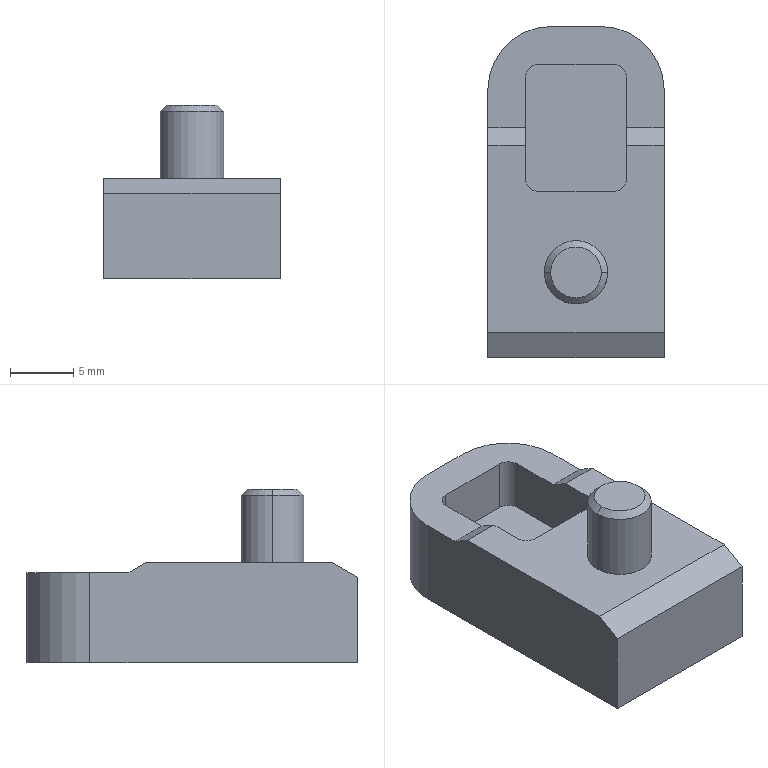Part | SolidWorks | features ICE 4, RefAxis 3, 3DProfileFeature 1, Extrusion 1, RevCut 1, Revolution 1 | 1 solid | 41 faces | box 13.9 x 26.1 x 13.7 mm | volume 2228 mm3 | plane 25 | cylinder 12 | cone 4 | commonest cylinder face diameters 2 x4 10 x4 5 x2 8.5 x2
STEP:
#1=CARTESIAN_POINT('',(2.5,6.7,7.9));
#2=VERTEX_POINT('',#1);
#3=CARTESIAN_POINT('',(-2.5,6.7,7.9));
#4=VERTEX_POINT('',#3);
#5=CARTESIAN_POINT('',(0.,6.7,7.9));
#6=DIRECTION('',(0.,0.,1.));
#7=DIRECTION('',(1.,0.,0.));
#8=AXIS2_PLACEMENT_3D('',#5,#6,#7);
#9=CIRCLE('',#8,2.5);
#10=EDGE_CURVE('',#2,#4,#9,.T.);
#11=ORIENTED_EDGE('',*,*,#10,.T.);
#12=CARTESIAN_POINT('',(-2.5,6.7,13.21));
#13=VERTEX_POINT('',#12);
#14=CARTESIAN_POINT('',(-2.5,6.7,7.9));
#15=DIRECTION('',(0.,0.,1.));
#16=VECTOR('',#15,1000.);
#17=LINE('',#14,#16);
#18=EDGE_CURVE('',#4,#13,#17,.T.);
#19=ORIENTED_EDGE('',*,*,#18,.T.);
#20=CARTESIAN_POINT('',(2.5,6.7,13.21));
#21=VERTEX_POINT('',#20);
#22=CARTESIAN_POINT('',(0.,6.7,13.21));
#23=DIRECTION('',(0.,0.,1.));
#24=DIRECTION('',(1.,0.,0.));
#25=AXIS2_PLACEMENT_3D('',#22,#23,#24);
#26=CIRCLE('',#25,2.5);
#27=EDGE_CURVE('',#21,#13,#26,.T.);
#28=ORIENTED_EDGE('',*,*,#27,.F.);
#29=CARTESIAN_POINT('',(2.5,6.7,7.9));
#30=DIRECTION('',(0.,0.,1.));
#31=VECTOR('',#30,1000.);
#32=LINE('',#29,#31);
#33=EDGE_CURVE('',#2,#21,#32,.T.);
#34=ORIENTED_EDGE('',*,*,#33,.F.);
#35=EDGE_LOOP('',(#11,#19,#28,#34));
#36=FACE_OUTER_BOUND('',#35,.T.);
#37=CARTESIAN_POINT('',(0.,6.7,7.9));
#38=DIRECTION('',(0.,0.,1.));
#39=DIRECTION('',(1.,0.,0.));
#40=AXIS2_PLACEMENT_3D('',#37,#38,#39);
#41=CYLINDRICAL_SURFACE('',#40,2.5);
#42=ADVANCED_FACE('',(#36),#41,.T.);
#43=CARTESIAN_POINT('',(2.01,6.7,13.7));
#44=VERTEX_POINT('',#43);
#45=CARTESIAN_POINT('',(-2.01,6.7,13.7));
#46=VERTEX_POINT('',#45);
#47=CARTESIAN_POINT('',(0.,6.7,13.7));
#48=DIRECTION('',(0.,0.,1.));
#49=DIRECTION('',(1.,0.,0.));
#50=AXIS2_PLACEMENT_3D('',#47,#48,#49);
#51=CIRCLE('',#50,2.01);
#52=EDGE_CURVE('',#44,#46,#51,.T.);
#53=ORIENTED_EDGE('',*,*,#52,.F.);
#54=CARTESIAN_POINT('',(2.5,6.7,13.21));
#55=DIRECTION('',(0.7071,0.,-0.7071));
#56=VECTOR('',#55,1000.);
#57=LINE('',#54,#56);
#58=EDGE_CURVE('',#44,#21,#57,.T.);
#59=ORIENTED_EDGE('',*,*,#58,.T.);
#60=ORIENTED_EDGE('',*,*,#27,.T.);
#61=CARTESIAN_POINT('',(-2.5,6.7,13.21));
#62=DIRECTION('',(-0.7071,0.,-0.7071));
#63=VECTOR('',#62,1000.);
#64=LINE('',#61,#63);
#65=EDGE_CURVE('',#46,#13,#64,.T.);
#66=ORIENTED_EDGE('',*,*,#65,.F.);
#67=EDGE_LOOP('',(#53,#59,#60,#66));
#68=FACE_OUTER_BOUND('',#67,.T.);
#69=CARTESIAN_POINT('',(0.,6.7,13.21));
#70=DIRECTION('',(0.,0.,-1.));
#71=DIRECTION('',(-1.,0.,0.));
#72=AXIS2_PLACEMENT_3D('',#69,#70,#71);
#73=CONICAL_SURFACE('',#72,2.5,0.7854);
#74=ADVANCED_FACE('',(#68),#73,.T.);
#75=CARTESIAN_POINT('',(-5.,6.7,0.));
#76=VERTEX_POINT('',#75);
#77=CARTESIAN_POINT('',(5.,6.7,0.));
#78=VERTEX_POINT('',#77);
#79=CARTESIAN_POINT('',(0.,6.7,0.));
#80=DIRECTION('',(0.,0.,1.));
#81=DIRECTION('',(1.,0.,0.));
#82=AXIS2_PLACEMENT_3D('',#79,#80,#81);
#83=CIRCLE('',#82,5.);
#84=EDGE_CURVE('',#76,#78,#83,.T.);
#85=ORIENTED_EDGE('',*,*,#84,.F.);
#86=CARTESIAN_POINT('',(-5.,6.7,5.7));
#87=VERTEX_POINT('',#86);
#88=CARTESIAN_POINT('',(-5.,6.7,0.));
#89=DIRECTION('',(0.,0.,1.));
#90=VECTOR('',#89,1000.);
#91=LINE('',#88,#90);
#92=EDGE_CURVE('',#76,#87,#91,.T.);
#93=ORIENTED_EDGE('',*,*,#92,.T.);
#94=CARTESIAN_POINT('',(5.,6.7,5.7));
#95=VERTEX_POINT('',#94);
#96=CARTESIAN_POINT('',(0.,6.7,5.7));
#97=DIRECTION('',(0.,0.,1.));
#98=DIRECTION('',(1.,0.,0.));
#99=AXIS2_PLACEMENT_3D('',#96,#97,#98);
#100=CIRCLE('',#99,5.);
#101=EDGE_CURVE('',#87,#95,#100,.T.);
#102=ORIENTED_EDGE('',*,*,#101,.T.);
#103=CARTESIAN_POINT('',(5.,6.7,0.));
#104=DIRECTION('',(0.,0.,1.));
#105=VECTOR('',#104,1000.);
#106=LINE('',#103,#105);
#107=EDGE_CURVE('',#78,#95,#106,.T.);
#108=ORIENTED_EDGE('',*,*,#107,.F.);
#109=EDGE_LOOP('',(#85,#93,#102,#108));
#110=FACE_OUTER_BOUND('',#109,.T.);
#111=CARTESIAN_POINT('',(0.,6.7,0.));
#112=DIRECTION('',(0.,0.,1.));
#113=DIRECTION('',(1.,0.,0.));
#114=AXIS2_PLACEMENT_3D('',#111,#112,#113);
#115=CYLINDRICAL_SURFACE('',#114,5.);
#116=ADVANCED_FACE('',(#110),#115,.F.);
#117=CARTESIAN_POINT('',(4.25,6.7,1.2));
#118=VERTEX_POINT('',#117);
#119=CARTESIAN_POINT('',(-4.25,6.7,1.2));
#120=VERTEX_POINT('',#119);
#121=CARTESIAN_POINT('',(0.,6.7,1.2));
#122=DIRECTION('',(0.,0.,1.));
#123=DIRECTION('',(1.,0.,0.));
#124=AXIS2_PLACEMENT_3D('',#121,#122,#123);
#125=CIRCLE('',#124,4.25);
#126=EDGE_CURVE('',#118,#120,#125,.T.);
#127=ORIENTED_EDGE('',*,*,#126,.T.);
#128=CARTESIAN_POINT('',(-4.25,6.7,5.7));
#129=VERTEX_POINT('',#128);
#130=CARTESIAN_POINT('',(-4.25,6.7,0.));
#131=DIRECTION('',(0.,0.,1.));
#132=VECTOR('',#131,1000.);
#133=LINE('',#130,#132);
#134=EDGE_CURVE('',#120,#129,#133,.T.);
#135=ORIENTED_EDGE('',*,*,#134,.T.);
#136=CARTESIAN_POINT('',(4.25,6.7,5.7));
#137=VERTEX_POINT('',#136);
#138=CARTESIAN_POINT('',(0.,6.7,5.7));
#139=DIRECTION('',(0.,0.,1.));
#140=DIRECTION('',(1.,0.,0.));
#141=AXIS2_PLACEMENT_3D('',#138,#139,#140);
#142=CIRCLE('',#141,4.25);
#143=EDGE_CURVE('',#137,#129,#142,.T.);
#144=ORIENTED_EDGE('',*,*,#143,.F.);
#145=CARTESIAN_POINT('',(4.25,6.7,0.));
#146=DIRECTION('',(0.,0.,1.));
#147=VECTOR('',#146,1000.);
#148=LINE('',#145,#147);
#149=EDGE_CURVE('',#118,#137,#148,.T.);
#150=ORIENTED_EDGE('',*,*,#149,.F.);
#151=EDGE_LOOP('',(#127,#135,#144,#150));
#152=FACE_OUTER_BOUND('',#151,.T.);
#153=CARTESIAN_POINT('',(0.,6.7,0.));
#154=DIRECTION('',(0.,0.,1.));
#155=DIRECTION('',(1.,0.,0.));
#156=AXIS2_PLACEMENT_3D('',#153,#154,#155);
#157=CYLINDRICAL_SURFACE('',#156,4.25);
#158=ADVANCED_FACE('',(#152),#157,.T.);
#159=CARTESIAN_POINT('',(3.75,6.7,0.7));
#160=VERTEX_POINT('',#159);
#161=CARTESIAN_POINT('',(-3.75,6.7,0.7));
#162=VERTEX_POINT('',#161);
#163=CARTESIAN_POINT('',(0.,6.7,0.7));
#164=DIRECTION('',(0.,0.,1.));
#165=DIRECTION('',(1.,0.,0.));
#166=AXIS2_PLACEMENT_3D('',#163,#164,#165);
#167=CIRCLE('',#166,3.75);
#168=EDGE_CURVE('',#160,#162,#167,.T.);
#169=ORIENTED_EDGE('',*,*,#168,.T.);
#170=CARTESIAN_POINT('',(-4.25,6.7,1.2));
#171=DIRECTION('',(-0.7071,0.,0.7071));
#172=VECTOR('',#171,1000.);
#173=LINE('',#170,#172);
#174=EDGE_CURVE('',#162,#120,#173,.T.);
#175=ORIENTED_EDGE('',*,*,#174,.T.);
#176=ORIENTED_EDGE('',*,*,#126,.F.);
#177=CARTESIAN_POINT('',(4.25,6.7,1.2));
#178=DIRECTION('',(0.7071,0.,0.7071));
#179=VECTOR('',#178,1000.);
#180=LINE('',#177,#179);
#181=EDGE_CURVE('',#160,#118,#180,.T.);
#182=ORIENTED_EDGE('',*,*,#181,.F.);
#183=EDGE_LOOP('',(#169,#175,#176,#182));
#184=FACE_OUTER_BOUND('',#183,.T.);
#185=CARTESIAN_POINT('',(0.,6.7,1.2));
#186=DIRECTION('',(0.,0.,1.));
#187=DIRECTION('',(1.,0.,0.));
#188=AXIS2_PLACEMENT_3D('',#185,#186,#187);
#189=CONICAL_SURFACE('',#188,4.25,0.7854);
#190=ADVANCED_FACE('',(#184),#189,.T.);
#191=CARTESIAN_POINT('',(4.,14.1,7.9));
#192=VERTEX_POINT('',#191);
#193=CARTESIAN_POINT('',(4.,16.714,7.9));
#194=VERTEX_POINT('',#193);
#195=CARTESIAN_POINT('',(4.,14.1,7.9));
#196=DIRECTION('',(0.,1.,0.));
#197=VECTOR('',#196,1000.);
#198=LINE('',#195,#197);
#199=EDGE_CURVE('',#192,#194,#198,.T.);
#200=ORIENTED_EDGE('',*,*,#199,.F.);
#201=CARTESIAN_POINT('',(3.,13.1,7.9));
#202=VERTEX_POINT('',#201);
#203=CARTESIAN_POINT('',(3.,14.1,7.9));
#204=DIRECTION('',(0.,0.,1.));
#205=DIRECTION('',(1.,0.,0.));
#206=AXIS2_PLACEMENT_3D('',#203,#204,#205);
#207=CIRCLE('',#206,1.);
#208=EDGE_CURVE('',#202,#192,#207,.T.);
#209=ORIENTED_EDGE('',*,*,#208,.F.);
#210=CARTESIAN_POINT('',(-3.,13.1,7.9));
#211=VERTEX_POINT('',#210);
#212=CARTESIAN_POINT('',(-3.,13.1,7.9));
#213=DIRECTION('',(1.,0.,0.));
#214=VECTOR('',#213,1000.);
#215=LINE('',#212,#214);
#216=EDGE_CURVE('',#211,#202,#215,.T.);
#217=ORIENTED_EDGE('',*,*,#216,.F.);
#218=CARTESIAN_POINT('',(-4.,14.1,7.9));
#219=VERTEX_POINT('',#218);
#220=CARTESIAN_POINT('',(-3.,14.1,7.9));
#221=DIRECTION('',(0.,0.,1.));
#222=DIRECTION('',(1.,0.,0.));
#223=AXIS2_PLACEMENT_3D('',#220,#221,#222);
#224=CIRCLE('',#223,1.);
#225=EDGE_CURVE('',#219,#211,#224,.T.);
#226=ORIENTED_EDGE('',*,*,#225,.F.);
#227=CARTESIAN_POINT('',(-4.,16.714,7.9));
#228=VERTEX_POINT('',#227);
#229=CARTESIAN_POINT('',(-4.,22.1,7.9));
#230=DIRECTION('',(0.,-1.,0.));
#231=VECTOR('',#230,1000.);
#232=LINE('',#229,#231);
#233=EDGE_CURVE('',#228,#219,#232,.T.);
#234=ORIENTED_EDGE('',*,*,#233,.F.);
#235=CARTESIAN_POINT('',(-6.95,16.714,7.9));
#236=VERTEX_POINT('',#235);
#237=CARTESIAN_POINT('',(-6.95,16.714,7.9));
#238=DIRECTION('',(1.,0.,0.));
#239=VECTOR('',#238,1000.);
#240=LINE('',#237,#239);
#241=EDGE_CURVE('',#236,#228,#240,.T.);
#242=ORIENTED_EDGE('',*,*,#241,.F.);
#243=CARTESIAN_POINT('',(-6.95,2.,7.9));
#244=VERTEX_POINT('',#243);
#245=CARTESIAN_POINT('',(-6.95,21.1,7.9));
#246=DIRECTION('',(0.,-1.,0.));
#247=VECTOR('',#246,1000.);
#248=LINE('',#245,#247);
#249=EDGE_CURVE('',#236,#244,#248,.T.);
#250=ORIENTED_EDGE('',*,*,#249,.T.);
#251=CARTESIAN_POINT('',(6.95,2.,7.9));
#252=VERTEX_POINT('',#251);
#253=CARTESIAN_POINT('',(-6.95,2.,7.9));
#254=DIRECTION('',(1.,0.,0.));
#255=VECTOR('',#254,1000.);
#256=LINE('',#253,#255);
#257=EDGE_CURVE('',#244,#252,#256,.T.);
#258=ORIENTED_EDGE('',*,*,#257,.T.);
#259=CARTESIAN_POINT('',(6.95,16.714,7.9));
#260=VERTEX_POINT('',#259);
#261=CARTESIAN_POINT('',(6.95,0.,7.9));
#262=DIRECTION('',(0.,1.,0.));
#263=VECTOR('',#262,1000.);
#264=LINE('',#261,#263);
#265=EDGE_CURVE('',#252,#260,#264,.T.);
#266=ORIENTED_EDGE('',*,*,#265,.T.);
#267=CARTESIAN_POINT('',(-6.95,16.714,7.9));
#268=DIRECTION('',(1.,0.,0.));
#269=VECTOR('',#268,1000.);
#270=LINE('',#267,#269);
#271=EDGE_CURVE('',#194,#260,#270,.T.);
#272=ORIENTED_EDGE('',*,*,#271,.F.);
#273=EDGE_LOOP('',(#200,#209,#217,#226,#234,#242,#250,#258,#266,#272));
#274=FACE_OUTER_BOUND('',#273,.T.);
#275=ORIENTED_EDGE('',*,*,#10,.F.);
#276=CARTESIAN_POINT('',(0.,6.7,7.9));
#277=DIRECTION('',(0.,0.,1.));
#278=DIRECTION('',(1.,0.,0.));
#279=AXIS2_PLACEMENT_3D('',#276,#277,#278);
#280=CIRCLE('',#279,2.5);
#281=EDGE_CURVE('',#4,#2,#280,.T.);
#282=ORIENTED_EDGE('',*,*,#281,.F.);
#283=EDGE_LOOP('',(#275,#282));
#284=FACE_BOUND('',#283,.T.);
#285=CARTESIAN_POINT('',(-1.95,21.1,7.9));
#286=DIRECTION('',(0.,0.,1.));
#287=DIRECTION('',(1.,0.,0.));
#288=AXIS2_PLACEMENT_3D('',#285,#286,#287);
#289=PLANE('',#288);
#290=ADVANCED_FACE('',(#274,#284),#289,.T.);
#291=CARTESIAN_POINT('',(-1.95,26.1,0.));
#292=VERTEX_POINT('',#291);
#293=CARTESIAN_POINT('',(-6.95,21.1,0.));
#294=VERTEX_POINT('',#293);
#295=CARTESIAN_POINT('',(-1.95,21.1,0.));
#296=DIRECTION('',(0.,0.,1.));
#297=DIRECTION('',(1.,0.,0.));
#298=AXIS2_PLACEMENT_3D('',#295,#296,#297);
#299=CIRCLE('',#298,5.);
#300=EDGE_CURVE('',#292,#294,#299,.T.);
#301=ORIENTED_EDGE('',*,*,#300,.F.);
#302=CARTESIAN_POINT('',(1.95,26.1,0.));
#303=VERTEX_POINT('',#302);
#304=CARTESIAN_POINT('',(1.95,26.1,0.));
#305=DIRECTION('',(-1.,0.,0.));
#306=VECTOR('',#305,1000.);
#307=LINE('',#304,#306);
#308=EDGE_CURVE('',#303,#292,#307,.T.);
#309=ORIENTED_EDGE('',*,*,#308,.F.);
#310=CARTESIAN_POINT('',(6.95,21.1,0.));
#311=VERTEX_POINT('',#310);
#312=CARTESIAN_POINT('',(1.95,21.1,0.));
#313=DIRECTION('',(0.,0.,1.));
#314=DIRECTION('',(1.,0.,0.));
#315=AXIS2_PLACEMENT_3D('',#312,#313,#314);
#316=CIRCLE('',#315,5.);
#317=EDGE_CURVE('',#311,#303,#316,.T.);
#318=ORIENTED_EDGE('',*,*,#317,.F.);
#319=CARTESIAN_POINT('',(6.95,0.,0.));
#320=VERTEX_POINT('',#319);
#321=CARTESIAN_POINT('',(6.95,0.,0.));
#322=DIRECTION('',(0.,1.,0.));
#323=VECTOR('',#322,1000.);
#324=LINE('',#321,#323);
#325=EDGE_CURVE('',#320,#311,#324,.T.);
#326=ORIENTED_EDGE('',*,*,#325,.F.);
#327=CARTESIAN_POINT('',(-6.95,0.,0.));
#328=VERTEX_POINT('',#327);
#329=CARTESIAN_POINT('',(-6.95,0.,0.));
#330=DIRECTION('',(1.,0.,0.));
#331=VECTOR('',#330,1000.);
#332=LINE('',#329,#331);
#333=EDGE_CURVE('',#328,#320,#332,.T.);
#334=ORIENTED_EDGE('',*,*,#333,.F.);
#335=CARTESIAN_POINT('',(-6.95,21.1,0.));
#336=DIRECTION('',(0.,-1.,0.));
#337=VECTOR('',#336,1000.);
#338=LINE('',#335,#337);
#339=EDGE_CURVE('',#294,#328,#338,.T.);
#340=ORIENTED_EDGE('',*,*,#339,.F.);
#341=EDGE_LOOP('',(#301,#309,#318,#326,#334,#340));
#342=FACE_OUTER_BOUND('',#341,.T.);
#343=CARTESIAN_POINT('',(0.,6.7,0.));
#344=DIRECTION('',(0.,0.,1.));
#345=DIRECTION('',(1.,0.,0.));
#346=AXIS2_PLACEMENT_3D('',#343,#344,#345);
#347=CIRCLE('',#346,5.);
#348=EDGE_CURVE('',#78,#76,#347,.T.);
#349=ORIENTED_EDGE('',*,*,#348,.T.);
#350=ORIENTED_EDGE('',*,*,#84,.T.);
#351=EDGE_LOOP('',(#349,#350));
#352=FACE_BOUND('',#351,.T.);
#353=CARTESIAN_POINT('',(-1.95,21.1,0.));
#354=DIRECTION('',(0.,0.,1.));
#355=DIRECTION('',(1.,0.,0.));
#356=AXIS2_PLACEMENT_3D('',#353,#354,#355);
#357=PLANE('',#356);
#358=ADVANCED_FACE('',(#342,#352),#357,.F.);
#359=CARTESIAN_POINT('',(4.,18.1,7.1));
#360=VERTEX_POINT('',#359);
#361=CARTESIAN_POINT('',(6.95,18.1,7.1));
#362=VERTEX_POINT('',#361);
#363=CARTESIAN_POINT('',(-6.95,18.1,7.1));
#364=DIRECTION('',(1.,0.,0.));
#365=VECTOR('',#364,1000.);
#366=LINE('',#363,#365);
#367=EDGE_CURVE('',#360,#362,#366,.T.);
#368=ORIENTED_EDGE('',*,*,#367,.F.);
#369=CARTESIAN_POINT('',(4.,16.714,7.9));
#370=DIRECTION('',(0.,-0.866,0.5));
#371=VECTOR('',#370,1000.);
#372=LINE('',#369,#371);
#373=EDGE_CURVE('',#360,#194,#372,.T.);
#374=ORIENTED_EDGE('',*,*,#373,.T.);
#375=ORIENTED_EDGE('',*,*,#271,.T.);
#376=CARTESIAN_POINT('',(6.95,16.714,7.9));
#377=DIRECTION('',(0.,0.866,-0.5));
#378=VECTOR('',#377,1000.);
#379=LINE('',#376,#378);
#380=EDGE_CURVE('',#260,#362,#379,.T.);
#381=ORIENTED_EDGE('',*,*,#380,.T.);
#382=EDGE_LOOP('',(#368,#374,#375,#381));
#383=FACE_OUTER_BOUND('',#382,.T.);
#384=CARTESIAN_POINT('',(-6.95,16.714,7.9));
#385=DIRECTION('',(0.,-0.5,-0.866));
#386=DIRECTION('',(0.,0.866,-0.5));
#387=AXIS2_PLACEMENT_3D('',#384,#385,#386);
#388=PLANE('',#387);
#389=ADVANCED_FACE('',(#383),#388,.F.);
#390=CARTESIAN_POINT('',(-6.95,21.1,7.1));
#391=VERTEX_POINT('',#390);
#392=CARTESIAN_POINT('',(-6.95,21.1,7.9));
#393=DIRECTION('',(0.,0.,-1.));
#394=VECTOR('',#393,1000.);
#395=LINE('',#392,#394);
#396=EDGE_CURVE('',#391,#294,#395,.T.);
#397=ORIENTED_EDGE('',*,*,#396,.F.);
#398=CARTESIAN_POINT('',(-1.95,26.1,7.1));
#399=VERTEX_POINT('',#398);
#400=CARTESIAN_POINT('',(-1.95,21.1,7.1));
#401=DIRECTION('',(0.,0.,-1.));
#402=DIRECTION('',(-1.,0.,0.));
#403=AXIS2_PLACEMENT_3D('',#400,#401,#402);
#404=CIRCLE('',#403,5.);
#405=EDGE_CURVE('',#391,#399,#404,.T.);
#406=ORIENTED_EDGE('',*,*,#405,.T.);
#407=CARTESIAN_POINT('',(-1.95,26.1,7.9));
#408=DIRECTION('',(0.,0.,-1.));
#409=VECTOR('',#408,1000.);
#410=LINE('',#407,#409);
#411=EDGE_CURVE('',#399,#292,#410,.T.);
#412=ORIENTED_EDGE('',*,*,#411,.T.);
#413=ORIENTED_EDGE('',*,*,#300,.T.);
#414=EDGE_LOOP('',(#397,#406,#412,#413));
#415=FACE_OUTER_BOUND('',#414,.T.);
#416=CARTESIAN_POINT('',(-1.95,21.1,7.9));
#417=DIRECTION('',(0.,0.,-1.));
#418=DIRECTION('',(-1.,0.,0.));
#419=AXIS2_PLACEMENT_3D('',#416,#417,#418);
#420=CYLINDRICAL_SURFACE('',#419,5.);
#421=ADVANCED_FACE('',(#415),#420,.T.);
#422=CARTESIAN_POINT('',(-6.95,18.1,7.1));
#423=VERTEX_POINT('',#422);
#424=CARTESIAN_POINT('',(-6.95,16.714,7.9));
#425=DIRECTION('',(0.,0.866,-0.5));
#426=VECTOR('',#425,1000.);
#427=LINE('',#424,#426);
#428=EDGE_CURVE('',#236,#423,#427,.T.);
#429=ORIENTED_EDGE('',*,*,#428,.T.);
#430=CARTESIAN_POINT('',(-6.95,18.1,7.1));
#431=DIRECTION('',(0.,1.,0.));
#432=VECTOR('',#431,1000.);
#433=LINE('',#430,#432);
#434=EDGE_CURVE('',#423,#391,#433,.T.);
#435=ORIENTED_EDGE('',*,*,#434,.T.);
#436=ORIENTED_EDGE('',*,*,#396,.T.);
#437=ORIENTED_EDGE('',*,*,#339,.T.);
#438=CARTESIAN_POINT('',(-6.95,0.,6.745));
#439=VERTEX_POINT('',#438);
#440=CARTESIAN_POINT('',(-6.95,0.,7.9));
#441=DIRECTION('',(0.,0.,-1.));
#442=VECTOR('',#441,1000.);
#443=LINE('',#440,#442);
#444=EDGE_CURVE('',#439,#328,#443,.T.);
#445=ORIENTED_EDGE('',*,*,#444,.F.);
#446=CARTESIAN_POINT('',(-6.95,0.,6.745));
#447=DIRECTION('',(0.,0.866,0.5));
#448=VECTOR('',#447,1000.);
#449=LINE('',#446,#448);
#450=EDGE_CURVE('',#439,#244,#449,.T.);
#451=ORIENTED_EDGE('',*,*,#450,.T.);
#452=ORIENTED_EDGE('',*,*,#249,.F.);
#453=EDGE_LOOP('',(#429,#435,#436,#437,#445,#451,#452));
#454=FACE_OUTER_BOUND('',#453,.T.);
#455=CARTESIAN_POINT('',(-6.95,21.1,7.9));
#456=DIRECTION('',(1.,0.,0.));
#457=DIRECTION('',(0.,0.,-1.));
#458=AXIS2_PLACEMENT_3D('',#455,#456,#457);
#459=PLANE('',#458);
#460=ADVANCED_FACE('',(#454),#459,.F.);
#461=CARTESIAN_POINT('',(6.95,0.,6.745));
#462=VERTEX_POINT('',#461);
#463=CARTESIAN_POINT('',(6.95,0.,7.9));
#464=DIRECTION('',(0.,0.,-1.));
#465=VECTOR('',#464,1000.);
#466=LINE('',#463,#465);
#467=EDGE_CURVE('',#462,#320,#466,.T.);
#468=ORIENTED_EDGE('',*,*,#467,.F.);
#469=CARTESIAN_POINT('',(-6.95,0.,6.745));
#470=DIRECTION('',(1.,0.,0.));
#471=VECTOR('',#470,1000.);
#472=LINE('',#469,#471);
#473=EDGE_CURVE('',#439,#462,#472,.T.);
#474=ORIENTED_EDGE('',*,*,#473,.F.);
#475=ORIENTED_EDGE('',*,*,#444,.T.);
#476=ORIENTED_EDGE('',*,*,#333,.T.);
#477=EDGE_LOOP('',(#468,#474,#475,#476));
#478=FACE_OUTER_BOUND('',#477,.T.);
#479=CARTESIAN_POINT('',(-6.95,0.,7.9));
#480=DIRECTION('',(0.,1.,0.));
#481=DIRECTION('',(0.,0.,1.));
#482=AXIS2_PLACEMENT_3D('',#479,#480,#481);
#483=PLANE('',#482);
#484=ADVANCED_FACE('',(#478),#483,.F.);
#485=CARTESIAN_POINT('',(6.95,21.1,7.1));
#486=VERTEX_POINT('',#485);
#487=CARTESIAN_POINT('',(6.95,21.1,7.9));
#488=DIRECTION('',(0.,0.,-1.));
#489=VECTOR('',#488,1000.);
#490=LINE('',#487,#489);
#491=EDGE_CURVE('',#486,#311,#490,.T.);
#492=ORIENTED_EDGE('',*,*,#491,.F.);
#493=CARTESIAN_POINT('',(6.95,18.1,7.1));
#494=DIRECTION('',(0.,1.,0.));
#495=VECTOR('',#494,1000.);
#496=LINE('',#493,#495);
#497=EDGE_CURVE('',#362,#486,#496,.T.);
#498=ORIENTED_EDGE('',*,*,#497,.F.);
#499=ORIENTED_EDGE('',*,*,#380,.F.);
#500=ORIENTED_EDGE('',*,*,#265,.F.);
#501=CARTESIAN_POINT('',(6.95,0.,6.745));
#502=DIRECTION('',(0.,0.866,0.5));
#503=VECTOR('',#502,1000.);
#504=LINE('',#501,#503);
#505=EDGE_CURVE('',#462,#252,#504,.T.);
#506=ORIENTED_EDGE('',*,*,#505,.F.);
#507=ORIENTED_EDGE('',*,*,#467,.T.);
#508=ORIENTED_EDGE('',*,*,#325,.T.);
#509=EDGE_LOOP('',(#492,#498,#499,#500,#506,#507,#508));
#510=FACE_OUTER_BOUND('',#509,.T.);
#511=CARTESIAN_POINT('',(6.95,0.,7.9));
#512=DIRECTION('',(-1.,0.,0.));
#513=DIRECTION('',(0.,0.,1.));
#514=AXIS2_PLACEMENT_3D('',#511,#512,#513);
#515=PLANE('',#514);
#516=ADVANCED_FACE('',(#510),#515,.F.);
#517=CARTESIAN_POINT('',(1.95,26.1,7.1));
#518=VERTEX_POINT('',#517);
#519=CARTESIAN_POINT('',(1.95,26.1,7.9));
#520=DIRECTION('',(0.,0.,-1.));
#521=VECTOR('',#520,1000.);
#522=LINE('',#519,#521);
#523=EDGE_CURVE('',#518,#303,#522,.T.);
#524=ORIENTED_EDGE('',*,*,#523,.F.);
#525=CARTESIAN_POINT('',(1.95,21.1,7.1));
#526=DIRECTION('',(0.,0.,-1.));
#527=DIRECTION('',(-1.,0.,0.));
#528=AXIS2_PLACEMENT_3D('',#525,#526,#527);
#529=CIRCLE('',#528,5.);
#530=EDGE_CURVE('',#518,#486,#529,.T.);
#531=ORIENTED_EDGE('',*,*,#530,.T.);
#532=ORIENTED_EDGE('',*,*,#491,.T.);
#533=ORIENTED_EDGE('',*,*,#317,.T.);
#534=EDGE_LOOP('',(#524,#531,#532,#533));
#535=FACE_OUTER_BOUND('',#534,.T.);
#536=CARTESIAN_POINT('',(1.95,21.1,7.9));
#537=DIRECTION('',(0.,0.,-1.));
#538=DIRECTION('',(-1.,0.,0.));
#539=AXIS2_PLACEMENT_3D('',#536,#537,#538);
#540=CYLINDRICAL_SURFACE('',#539,5.);
#541=ADVANCED_FACE('',(#535),#540,.T.);
#542=ORIENTED_EDGE('',*,*,#411,.F.);
#543=CARTESIAN_POINT('',(-6.95,26.1,7.1));
#544=DIRECTION('',(1.,0.,0.));
#545=VECTOR('',#544,1000.);
#546=LINE('',#543,#545);
#547=EDGE_CURVE('',#399,#518,#546,.T.);
#548=ORIENTED_EDGE('',*,*,#547,.T.);
#549=ORIENTED_EDGE('',*,*,#523,.T.);
#550=ORIENTED_EDGE('',*,*,#308,.T.);
#551=EDGE_LOOP('',(#542,#548,#549,#550));
#552=FACE_OUTER_BOUND('',#551,.T.);
#553=CARTESIAN_POINT('',(1.95,26.1,7.9));
#554=DIRECTION('',(0.,-1.,0.));
#555=DIRECTION('',(0.,0.,-1.));
#556=AXIS2_PLACEMENT_3D('',#553,#554,#555);
#557=PLANE('',#556);
#558=ADVANCED_FACE('',(#552),#557,.F.);
#559=ORIENTED_EDGE('',*,*,#257,.F.);
#560=ORIENTED_EDGE('',*,*,#450,.F.);
#561=ORIENTED_EDGE('',*,*,#473,.T.);
#562=ORIENTED_EDGE('',*,*,#505,.T.);
#563=EDGE_LOOP('',(#559,#560,#561,#562));
#564=FACE_OUTER_BOUND('',#563,.T.);
#565=CARTESIAN_POINT('',(-6.95,0.,6.745));
#566=DIRECTION('',(0.,0.5,-0.866));
#567=DIRECTION('',(0.,0.866,0.5));
#568=AXIS2_PLACEMENT_3D('',#565,#566,#567);
#569=PLANE('',#568);
#570=ADVANCED_FACE('',(#564),#569,.F.);
#571=CARTESIAN_POINT('',(3.,23.1,7.1));
#572=VERTEX_POINT('',#571);
#573=CARTESIAN_POINT('',(4.,22.1,7.1));
#574=VERTEX_POINT('',#573);
#575=CARTESIAN_POINT('',(3.,22.1,7.1));
#576=DIRECTION('',(0.,0.,-1.));
#577=DIRECTION('',(-1.,0.,0.));
#578=AXIS2_PLACEMENT_3D('',#575,#576,#577);
#579=CIRCLE('',#578,1.);
#580=EDGE_CURVE('',#572,#574,#579,.T.);
#581=ORIENTED_EDGE('',*,*,#580,.T.);
#582=CARTESIAN_POINT('',(4.,18.1,7.1));
#583=DIRECTION('',(0.,-1.,0.));
#584=VECTOR('',#583,1000.);
#585=LINE('',#582,#584);
#586=EDGE_CURVE('',#574,#360,#585,.T.);
#587=ORIENTED_EDGE('',*,*,#586,.T.);
#588=ORIENTED_EDGE('',*,*,#367,.T.);
#589=ORIENTED_EDGE('',*,*,#497,.T.);
#590=ORIENTED_EDGE('',*,*,#530,.F.);
#591=ORIENTED_EDGE('',*,*,#547,.F.);
#592=ORIENTED_EDGE('',*,*,#405,.F.);
#593=ORIENTED_EDGE('',*,*,#434,.F.);
#594=CARTESIAN_POINT('',(-4.,18.1,7.1));
#595=VERTEX_POINT('',#594);
#596=CARTESIAN_POINT('',(-6.95,18.1,7.1));
#597=DIRECTION('',(1.,0.,0.));
#598=VECTOR('',#597,1000.);
#599=LINE('',#596,#598);
#600=EDGE_CURVE('',#423,#595,#599,.T.);
#601=ORIENTED_EDGE('',*,*,#600,.T.);
#602=CARTESIAN_POINT('',(-4.,22.1,7.1));
#603=VERTEX_POINT('',#602);
#604=CARTESIAN_POINT('',(-4.,18.1,7.1));
#605=DIRECTION('',(0.,1.,0.));
#606=VECTOR('',#605,1000.);
#607=LINE('',#604,#606);
#608=EDGE_CURVE('',#595,#603,#607,.T.);
#609=ORIENTED_EDGE('',*,*,#608,.T.);
#610=CARTESIAN_POINT('',(-3.,23.1,7.1));
#611=VERTEX_POINT('',#610);
#612=CARTESIAN_POINT('',(-3.,22.1,7.1));
#613=DIRECTION('',(0.,0.,-1.));
#614=DIRECTION('',(-1.,0.,0.));
#615=AXIS2_PLACEMENT_3D('',#612,#613,#614);
#616=CIRCLE('',#615,1.);
#617=EDGE_CURVE('',#603,#611,#616,.T.);
#618=ORIENTED_EDGE('',*,*,#617,.T.);
#619=CARTESIAN_POINT('',(-6.95,23.1,7.1));
#620=DIRECTION('',(1.,0.,0.));
#621=VECTOR('',#620,1000.);
#622=LINE('',#619,#621);
#623=EDGE_CURVE('',#611,#572,#622,.T.);
#624=ORIENTED_EDGE('',*,*,#623,.T.);
#625=EDGE_LOOP('',(#581,#587,#588,#589,#590,#591,#592,#593,#601,#609,#618,#624));
#626=FACE_OUTER_BOUND('',#625,.T.);
#627=CARTESIAN_POINT('',(-6.95,18.1,7.1));
#628=DIRECTION('',(0.,0.,-1.));
#629=DIRECTION('',(-1.,0.,0.));
#630=AXIS2_PLACEMENT_3D('',#627,#628,#629);
#631=PLANE('',#630);
#632=ADVANCED_FACE('',(#626),#631,.F.);
#633=ORIENTED_EDGE('',*,*,#241,.T.);
#634=CARTESIAN_POINT('',(-4.,16.714,7.9));
#635=DIRECTION('',(0.,0.866,-0.5));
#636=VECTOR('',#635,1000.);
#637=LINE('',#634,#636);
#638=EDGE_CURVE('',#228,#595,#637,.T.);
#639=ORIENTED_EDGE('',*,*,#638,.T.);
#640=ORIENTED_EDGE('',*,*,#600,.F.);
#641=ORIENTED_EDGE('',*,*,#428,.F.);
#642=EDGE_LOOP('',(#633,#639,#640,#641));
#643=FACE_OUTER_BOUND('',#642,.T.);
#644=CARTESIAN_POINT('',(-6.95,16.714,7.9));
#645=DIRECTION('',(0.,-0.5,-0.866));
#646=DIRECTION('',(0.,0.866,-0.5));
#647=AXIS2_PLACEMENT_3D('',#644,#645,#646);
#648=PLANE('',#647);
#649=ADVANCED_FACE('',(#643),#648,.F.);
#650=CARTESIAN_POINT('',(-4.,22.1,2.9));
#651=VERTEX_POINT('',#650);
#652=CARTESIAN_POINT('',(-4.,22.1,2.9));
#653=DIRECTION('',(0.,0.,1.));
#654=VECTOR('',#653,1000.);
#655=LINE('',#652,#654);
#656=EDGE_CURVE('',#651,#603,#655,.T.);
#657=ORIENTED_EDGE('',*,*,#656,.F.);
#658=CARTESIAN_POINT('',(-3.,23.1,2.9));
#659=VERTEX_POINT('',#658);
#660=CARTESIAN_POINT('',(-3.,22.1,2.9));
#661=DIRECTION('',(0.,0.,1.));
#662=DIRECTION('',(1.,0.,0.));
#663=AXIS2_PLACEMENT_3D('',#660,#661,#662);
#664=CIRCLE('',#663,1.);
#665=EDGE_CURVE('',#659,#651,#664,.T.);
#666=ORIENTED_EDGE('',*,*,#665,.F.);
#667=CARTESIAN_POINT('',(-3.,23.1,2.9));
#668=DIRECTION('',(0.,0.,1.));
#669=VECTOR('',#668,1000.);
#670=LINE('',#667,#669);
#671=EDGE_CURVE('',#659,#611,#670,.T.);
#672=ORIENTED_EDGE('',*,*,#671,.T.);
#673=ORIENTED_EDGE('',*,*,#617,.F.);
#674=EDGE_LOOP('',(#657,#666,#672,#673));
#675=FACE_OUTER_BOUND('',#674,.T.);
#676=CARTESIAN_POINT('',(-3.,22.1,2.9));
#677=DIRECTION('',(0.,0.,1.));
#678=DIRECTION('',(1.,0.,0.));
#679=AXIS2_PLACEMENT_3D('',#676,#677,#678);
#680=CYLINDRICAL_SURFACE('',#679,1.);
#681=ADVANCED_FACE('',(#675),#680,.F.);
#682=ORIENTED_EDGE('',*,*,#671,.F.);
#683=CARTESIAN_POINT('',(3.,23.1,2.9));
#684=VERTEX_POINT('',#683);
#685=CARTESIAN_POINT('',(3.,23.1,2.9));
#686=DIRECTION('',(-1.,0.,0.));
#687=VECTOR('',#686,1000.);
#688=LINE('',#685,#687);
#689=EDGE_CURVE('',#684,#659,#688,.T.);
#690=ORIENTED_EDGE('',*,*,#689,.F.);
#691=CARTESIAN_POINT('',(3.,23.1,2.9));
#692=DIRECTION('',(0.,0.,1.));
#693=VECTOR('',#692,1000.);
#694=LINE('',#691,#693);
#695=EDGE_CURVE('',#684,#572,#694,.T.);
#696=ORIENTED_EDGE('',*,*,#695,.T.);
#697=ORIENTED_EDGE('',*,*,#623,.F.);
#698=EDGE_LOOP('',(#682,#690,#696,#697));
#699=FACE_OUTER_BOUND('',#698,.T.);
#700=CARTESIAN_POINT('',(3.,23.1,2.9));
#701=DIRECTION('',(0.,1.,0.));
#702=DIRECTION('',(0.,0.,1.));
#703=AXIS2_PLACEMENT_3D('',#700,#701,#702);
#704=PLANE('',#703);
#705=ADVANCED_FACE('',(#699),#704,.F.);
#706=ORIENTED_EDGE('',*,*,#695,.F.);
#707=CARTESIAN_POINT('',(4.,22.1,2.9));
#708=VERTEX_POINT('',#707);
#709=CARTESIAN_POINT('',(3.,22.1,2.9));
#710=DIRECTION('',(0.,0.,1.));
#711=DIRECTION('',(1.,0.,0.));
#712=AXIS2_PLACEMENT_3D('',#709,#710,#711);
#713=CIRCLE('',#712,1.);
#714=EDGE_CURVE('',#708,#684,#713,.T.);
#715=ORIENTED_EDGE('',*,*,#714,.F.);
#716=CARTESIAN_POINT('',(4.,22.1,2.9));
#717=DIRECTION('',(0.,0.,1.));
#718=VECTOR('',#717,1000.);
#719=LINE('',#716,#718);
#720=EDGE_CURVE('',#708,#574,#719,.T.);
#721=ORIENTED_EDGE('',*,*,#720,.T.);
#722=ORIENTED_EDGE('',*,*,#580,.F.);
#723=EDGE_LOOP('',(#706,#715,#721,#722));
#724=FACE_OUTER_BOUND('',#723,.T.);
#725=CARTESIAN_POINT('',(3.,22.1,2.9));
#726=DIRECTION('',(0.,0.,1.));
#727=DIRECTION('',(1.,0.,0.));
#728=AXIS2_PLACEMENT_3D('',#725,#726,#727);
#729=CYLINDRICAL_SURFACE('',#728,1.);
#730=ADVANCED_FACE('',(#724),#729,.F.);
#731=ORIENTED_EDGE('',*,*,#720,.F.);
#732=CARTESIAN_POINT('',(4.,14.1,2.9));
#733=VERTEX_POINT('',#732);
#734=CARTESIAN_POINT('',(4.,14.1,2.9));
#735=DIRECTION('',(0.,1.,0.));
#736=VECTOR('',#735,1000.);
#737=LINE('',#734,#736);
#738=EDGE_CURVE('',#733,#708,#737,.T.);
#739=ORIENTED_EDGE('',*,*,#738,.F.);
#740=CARTESIAN_POINT('',(4.,14.1,2.9));
#741=DIRECTION('',(0.,0.,1.));
#742=VECTOR('',#741,1000.);
#743=LINE('',#740,#742);
#744=EDGE_CURVE('',#733,#192,#743,.T.);
#745=ORIENTED_EDGE('',*,*,#744,.T.);
#746=ORIENTED_EDGE('',*,*,#199,.T.);
#747=ORIENTED_EDGE('',*,*,#373,.F.);
#748=ORIENTED_EDGE('',*,*,#586,.F.);
#749=EDGE_LOOP('',(#731,#739,#745,#746,#747,#748));
#750=FACE_OUTER_BOUND('',#749,.T.);
#751=CARTESIAN_POINT('',(4.,14.1,2.9));
#752=DIRECTION('',(1.,0.,0.));
#753=DIRECTION('',(0.,0.,-1.));
#754=AXIS2_PLACEMENT_3D('',#751,#752,#753);
#755=PLANE('',#754);
#756=ADVANCED_FACE('',(#750),#755,.F.);
#757=ORIENTED_EDGE('',*,*,#638,.F.);
#758=ORIENTED_EDGE('',*,*,#233,.T.);
#759=CARTESIAN_POINT('',(-4.,14.1,2.9));
#760=VERTEX_POINT('',#759);
#761=CARTESIAN_POINT('',(-4.,14.1,2.9));
#762=DIRECTION('',(0.,0.,1.));
#763=VECTOR('',#762,1000.);
#764=LINE('',#761,#763);
#765=EDGE_CURVE('',#760,#219,#764,.T.);
#766=ORIENTED_EDGE('',*,*,#765,.F.);
#767=CARTESIAN_POINT('',(-4.,22.1,2.9));
#768=DIRECTION('',(0.,-1.,0.));
#769=VECTOR('',#768,1000.);
#770=LINE('',#767,#769);
#771=EDGE_CURVE('',#651,#760,#770,.T.);
#772=ORIENTED_EDGE('',*,*,#771,.F.);
#773=ORIENTED_EDGE('',*,*,#656,.T.);
#774=ORIENTED_EDGE('',*,*,#608,.F.);
#775=EDGE_LOOP('',(#757,#758,#766,#772,#773,#774));
#776=FACE_OUTER_BOUND('',#775,.T.);
#777=CARTESIAN_POINT('',(-4.,22.1,2.9));
#778=DIRECTION('',(-1.,0.,0.));
#779=DIRECTION('',(0.,0.,1.));
#780=AXIS2_PLACEMENT_3D('',#777,#778,#779);
#781=PLANE('',#780);
#782=ADVANCED_FACE('',(#776),#781,.F.);
#783=ORIENTED_EDGE('',*,*,#208,.T.);
#784=ORIENTED_EDGE('',*,*,#744,.F.);
#785=CARTESIAN_POINT('',(3.,13.1,2.9));
#786=VERTEX_POINT('',#785);
#787=CARTESIAN_POINT('',(3.,14.1,2.9));
#788=DIRECTION('',(0.,0.,1.));
#789=DIRECTION('',(1.,0.,0.));
#790=AXIS2_PLACEMENT_3D('',#787,#788,#789);
#791=CIRCLE('',#790,1.);
#792=EDGE_CURVE('',#786,#733,#791,.T.);
#793=ORIENTED_EDGE('',*,*,#792,.F.);
#794=CARTESIAN_POINT('',(3.,13.1,2.9));
#795=DIRECTION('',(0.,0.,1.));
#796=VECTOR('',#795,1000.);
#797=LINE('',#794,#796);
#798=EDGE_CURVE('',#786,#202,#797,.T.);
#799=ORIENTED_EDGE('',*,*,#798,.T.);
#800=EDGE_LOOP('',(#783,#784,#793,#799));
#801=FACE_OUTER_BOUND('',#800,.T.);
#802=CARTESIAN_POINT('',(3.,14.1,2.9));
#803=DIRECTION('',(0.,0.,1.));
#804=DIRECTION('',(1.,0.,0.));
#805=AXIS2_PLACEMENT_3D('',#802,#803,#804);
#806=CYLINDRICAL_SURFACE('',#805,1.);
#807=ADVANCED_FACE('',(#801),#806,.F.);
#808=ORIENTED_EDGE('',*,*,#216,.T.);
#809=ORIENTED_EDGE('',*,*,#798,.F.);
#810=CARTESIAN_POINT('',(-3.,13.1,2.9));
#811=VERTEX_POINT('',#810);
#812=CARTESIAN_POINT('',(-3.,13.1,2.9));
#813=DIRECTION('',(1.,0.,0.));
#814=VECTOR('',#813,1000.);
#815=LINE('',#812,#814);
#816=EDGE_CURVE('',#811,#786,#815,.T.);
#817=ORIENTED_EDGE('',*,*,#816,.F.);
#818=CARTESIAN_POINT('',(-3.,13.1,2.9));
#819=DIRECTION('',(0.,0.,1.));
#820=VECTOR('',#819,1000.);
#821=LINE('',#818,#820);
#822=EDGE_CURVE('',#811,#211,#821,.T.);
#823=ORIENTED_EDGE('',*,*,#822,.T.);
#824=EDGE_LOOP('',(#808,#809,#817,#823));
#825=FACE_OUTER_BOUND('',#824,.T.);
#826=CARTESIAN_POINT('',(-3.,13.1,2.9));
#827=DIRECTION('',(0.,-1.,0.));
#828=DIRECTION('',(0.,0.,-1.));
#829=AXIS2_PLACEMENT_3D('',#826,#827,#828);
#830=PLANE('',#829);
#831=ADVANCED_FACE('',(#825),#830,.F.);
#832=ORIENTED_EDGE('',*,*,#225,.T.);
#833=ORIENTED_EDGE('',*,*,#822,.F.);
#834=CARTESIAN_POINT('',(-3.,14.1,2.9));
#835=DIRECTION('',(0.,0.,1.));
#836=DIRECTION('',(1.,0.,0.));
#837=AXIS2_PLACEMENT_3D('',#834,#835,#836);
#838=CIRCLE('',#837,1.);
#839=EDGE_CURVE('',#760,#811,#838,.T.);
#840=ORIENTED_EDGE('',*,*,#839,.F.);
#841=ORIENTED_EDGE('',*,*,#765,.T.);
#842=EDGE_LOOP('',(#832,#833,#840,#841));
#843=FACE_OUTER_BOUND('',#842,.T.);
#844=CARTESIAN_POINT('',(-3.,14.1,2.9));
#845=DIRECTION('',(0.,0.,1.));
#846=DIRECTION('',(1.,0.,0.));
#847=AXIS2_PLACEMENT_3D('',#844,#845,#846);
#848=CYLINDRICAL_SURFACE('',#847,1.);
#849=ADVANCED_FACE('',(#843),#848,.F.);
#850=ORIENTED_EDGE('',*,*,#665,.T.);
#851=ORIENTED_EDGE('',*,*,#771,.T.);
#852=ORIENTED_EDGE('',*,*,#839,.T.);
#853=ORIENTED_EDGE('',*,*,#816,.T.);
#854=ORIENTED_EDGE('',*,*,#792,.T.);
#855=ORIENTED_EDGE('',*,*,#738,.T.);
#856=ORIENTED_EDGE('',*,*,#714,.T.);
#857=ORIENTED_EDGE('',*,*,#689,.T.);
#858=EDGE_LOOP('',(#850,#851,#852,#853,#854,#855,#856,#857));
#859=FACE_OUTER_BOUND('',#858,.T.);
#860=CARTESIAN_POINT('',(-3.,22.1,2.9));
#861=DIRECTION('',(0.,0.,1.));
#862=DIRECTION('',(1.,0.,0.));
#863=AXIS2_PLACEMENT_3D('',#860,#861,#862);
#864=PLANE('',#863);
#865=ADVANCED_FACE('',(#859),#864,.T.);
#866=CARTESIAN_POINT('',(1.155,4.7,0.7));
#867=VERTEX_POINT('',#866);
#868=CARTESIAN_POINT('',(-1.155,4.7,0.7));
#869=VERTEX_POINT('',#868);
#870=CARTESIAN_POINT('',(1.155,4.7,0.7));
#871=DIRECTION('',(-1.,0.,0.));
#872=VECTOR('',#871,1000.);
#873=LINE('',#870,#872);
#874=EDGE_CURVE('',#867,#869,#873,.T.);
#875=ORIENTED_EDGE('',*,*,#874,.F.);
#876=CARTESIAN_POINT('',(2.309,6.7,0.7));
#877=VERTEX_POINT('',#876);
#878=CARTESIAN_POINT('',(2.309,6.7,0.7));
#879=DIRECTION('',(-0.5,-0.866,0.));
#880=VECTOR('',#879,1000.);
#881=LINE('',#878,#880);
#882=EDGE_CURVE('',#877,#867,#881,.T.);
#883=ORIENTED_EDGE('',*,*,#882,.F.);
#884=CARTESIAN_POINT('',(1.155,8.7,0.7));
#885=VERTEX_POINT('',#884);
#886=CARTESIAN_POINT('',(1.155,8.7,0.7));
#887=DIRECTION('',(0.5,-0.866,0.));
#888=VECTOR('',#887,1000.);
#889=LINE('',#886,#888);
#890=EDGE_CURVE('',#885,#877,#889,.T.);
#891=ORIENTED_EDGE('',*,*,#890,.F.);
#892=CARTESIAN_POINT('',(-1.155,8.7,0.7));
#893=VERTEX_POINT('',#892);
#894=CARTESIAN_POINT('',(-1.155,8.7,0.7));
#895=DIRECTION('',(1.,0.,0.));
#896=VECTOR('',#895,1000.);
#897=LINE('',#894,#896);
#898=EDGE_CURVE('',#893,#885,#897,.T.);
#899=ORIENTED_EDGE('',*,*,#898,.F.);
#900=CARTESIAN_POINT('',(-2.309,6.7,0.7));
#901=VERTEX_POINT('',#900);
#902=CARTESIAN_POINT('',(-2.309,6.7,0.7));
#903=DIRECTION('',(0.5,0.866,0.));
#904=VECTOR('',#903,1000.);
#905=LINE('',#902,#904);
#906=EDGE_CURVE('',#901,#893,#905,.T.);
#907=ORIENTED_EDGE('',*,*,#906,.F.);
#908=CARTESIAN_POINT('',(-1.155,4.7,0.7));
#909=DIRECTION('',(-0.5,0.866,0.));
#910=VECTOR('',#909,1000.);
#911=LINE('',#908,#910);
#912=EDGE_CURVE('',#869,#901,#911,.T.);
#913=ORIENTED_EDGE('',*,*,#912,.F.);
#914=EDGE_LOOP('',(#875,#883,#891,#899,#907,#913));
#915=FACE_BOUND('',#914,.T.);
#916=ORIENTED_EDGE('',*,*,#168,.F.);
#917=CARTESIAN_POINT('',(0.,6.7,0.7));
#918=DIRECTION('',(0.,0.,1.));
#919=DIRECTION('',(1.,0.,0.));
#920=AXIS2_PLACEMENT_3D('',#917,#918,#919);
#921=CIRCLE('',#920,3.75);
#922=EDGE_CURVE('',#162,#160,#921,.T.);
#923=ORIENTED_EDGE('',*,*,#922,.F.);
#924=EDGE_LOOP('',(#916,#923));
#925=FACE_OUTER_BOUND('',#924,.T.);
#926=CARTESIAN_POINT('',(0.,6.7,0.7));
#927=DIRECTION('',(0.,0.,-1.));
#928=DIRECTION('',(-1.,0.,0.));
#929=AXIS2_PLACEMENT_3D('',#926,#927,#928);
#930=PLANE('',#929);
#931=ADVANCED_FACE('',(#915,#925),#930,.T.);
#932=ORIENTED_EDGE('',*,*,#174,.F.);
#933=ORIENTED_EDGE('',*,*,#922,.T.);
#934=ORIENTED_EDGE('',*,*,#181,.T.);
#935=CARTESIAN_POINT('',(0.,6.7,1.2));
#936=DIRECTION('',(0.,0.,1.));
#937=DIRECTION('',(1.,0.,0.));
#938=AXIS2_PLACEMENT_3D('',#935,#936,#937);
#939=CIRCLE('',#938,4.25);
#940=EDGE_CURVE('',#120,#118,#939,.T.);
#941=ORIENTED_EDGE('',*,*,#940,.F.);
#942=EDGE_LOOP('',(#932,#933,#934,#941));
#943=FACE_OUTER_BOUND('',#942,.T.);
#944=CARTESIAN_POINT('',(0.,6.7,1.2));
#945=DIRECTION('',(0.,0.,1.));
#946=DIRECTION('',(1.,0.,0.));
#947=AXIS2_PLACEMENT_3D('',#944,#945,#946);
#948=CONICAL_SURFACE('',#947,4.25,0.7854);
#949=ADVANCED_FACE('',(#943),#948,.T.);
#950=ORIENTED_EDGE('',*,*,#134,.F.);
#951=ORIENTED_EDGE('',*,*,#940,.T.);
#952=ORIENTED_EDGE('',*,*,#149,.T.);
#953=CARTESIAN_POINT('',(0.,6.7,5.7));
#954=DIRECTION('',(0.,0.,1.));
#955=DIRECTION('',(1.,0.,0.));
#956=AXIS2_PLACEMENT_3D('',#953,#954,#955);
#957=CIRCLE('',#956,4.25);
#958=EDGE_CURVE('',#129,#137,#957,.T.);
#959=ORIENTED_EDGE('',*,*,#958,.F.);
#960=EDGE_LOOP('',(#950,#951,#952,#959));
#961=FACE_OUTER_BOUND('',#960,.T.);
#962=CARTESIAN_POINT('',(0.,6.7,0.));
#963=DIRECTION('',(0.,0.,1.));
#964=DIRECTION('',(1.,0.,0.));
#965=AXIS2_PLACEMENT_3D('',#962,#963,#964);
#966=CYLINDRICAL_SURFACE('',#965,4.25);
#967=ADVANCED_FACE('',(#961),#966,.T.);
#968=ORIENTED_EDGE('',*,*,#143,.T.);
#969=ORIENTED_EDGE('',*,*,#958,.T.);
#970=EDGE_LOOP('',(#968,#969));
#971=FACE_BOUND('',#970,.T.);
#972=CARTESIAN_POINT('',(0.,6.7,5.7));
#973=DIRECTION('',(0.,0.,1.));
#974=DIRECTION('',(1.,0.,0.));
#975=AXIS2_PLACEMENT_3D('',#972,#973,#974);
#976=CIRCLE('',#975,5.);
#977=EDGE_CURVE('',#95,#87,#976,.T.);
#978=ORIENTED_EDGE('',*,*,#977,.F.);
#979=ORIENTED_EDGE('',*,*,#101,.F.);
#980=EDGE_LOOP('',(#978,#979));
#981=FACE_OUTER_BOUND('',#980,.T.);
#982=CARTESIAN_POINT('',(0.,10.95,5.7));
#983=DIRECTION('',(0.,0.,-1.));
#984=DIRECTION('',(-1.,0.,0.));
#985=AXIS2_PLACEMENT_3D('',#982,#983,#984);
#986=PLANE('',#985);
#987=ADVANCED_FACE('',(#971,#981),#986,.T.);
#988=ORIENTED_EDGE('',*,*,#92,.F.);
#989=ORIENTED_EDGE('',*,*,#348,.F.);
#990=ORIENTED_EDGE('',*,*,#107,.T.);
#991=ORIENTED_EDGE('',*,*,#977,.T.);
#992=EDGE_LOOP('',(#988,#989,#990,#991));
#993=FACE_OUTER_BOUND('',#992,.T.);
#994=CARTESIAN_POINT('',(0.,6.7,0.));
#995=DIRECTION('',(0.,0.,1.));
#996=DIRECTION('',(1.,0.,0.));
#997=AXIS2_PLACEMENT_3D('',#994,#995,#996);
#998=CYLINDRICAL_SURFACE('',#997,5.);
#999=ADVANCED_FACE('',(#993),#998,.F.);
#1000=ORIENTED_EDGE('',*,*,#874,.T.);
#1001=CARTESIAN_POINT('',(-1.155,4.7,3.2));
#1002=VERTEX_POINT('',#1001);
#1003=CARTESIAN_POINT('',(-1.155,4.7,3.2));
#1004=DIRECTION('',(0.,0.,-1.));
#1005=VECTOR('',#1004,1000.);
#1006=LINE('',#1003,#1005);
#1007=EDGE_CURVE('',#1002,#869,#1006,.T.);
#1008=ORIENTED_EDGE('',*,*,#1007,.F.);
#1009=CARTESIAN_POINT('',(1.155,4.7,3.2));
#1010=VERTEX_POINT('',#1009);
#1011=CARTESIAN_POINT('',(1.155,4.7,3.2));
#1012=DIRECTION('',(-1.,0.,0.));
#1013=VECTOR('',#1012,1000.);
#1014=LINE('',#1011,#1013);
#1015=EDGE_CURVE('',#1010,#1002,#1014,.T.);
#1016=ORIENTED_EDGE('',*,*,#1015,.F.);
#1017=CARTESIAN_POINT('',(1.155,4.7,3.2));
#1018=DIRECTION('',(0.,0.,-1.));
#1019=VECTOR('',#1018,1000.);
#1020=LINE('',#1017,#1019);
#1021=EDGE_CURVE('',#1010,#867,#1020,.T.);
#1022=ORIENTED_EDGE('',*,*,#1021,.T.);
#1023=EDGE_LOOP('',(#1000,#1008,#1016,#1022));
#1024=FACE_OUTER_BOUND('',#1023,.T.);
#1025=CARTESIAN_POINT('',(1.155,4.7,3.2));
#1026=DIRECTION('',(0.,-1.,0.));
#1027=DIRECTION('',(0.,0.,-1.));
#1028=AXIS2_PLACEMENT_3D('',#1025,#1026,#1027);
#1029=PLANE('',#1028);
#1030=ADVANCED_FACE('',(#1024),#1029,.F.);
#1031=ORIENTED_EDGE('',*,*,#882,.T.);
#1032=ORIENTED_EDGE('',*,*,#1021,.F.);
#1033=CARTESIAN_POINT('',(2.309,6.7,3.2));
#1034=VERTEX_POINT('',#1033);
#1035=CARTESIAN_POINT('',(2.309,6.7,3.2));
#1036=DIRECTION('',(-0.5,-0.866,0.));
#1037=VECTOR('',#1036,1000.);
#1038=LINE('',#1035,#1037);
#1039=EDGE_CURVE('',#1034,#1010,#1038,.T.);
#1040=ORIENTED_EDGE('',*,*,#1039,.F.);
#1041=CARTESIAN_POINT('',(2.309,6.7,3.2));
#1042=DIRECTION('',(0.,0.,-1.));
#1043=VECTOR('',#1042,1000.);
#1044=LINE('',#1041,#1043);
#1045=EDGE_CURVE('',#1034,#877,#1044,.T.);
#1046=ORIENTED_EDGE('',*,*,#1045,.T.);
#1047=EDGE_LOOP('',(#1031,#1032,#1040,#1046));
#1048=FACE_OUTER_BOUND('',#1047,.T.);
#1049=CARTESIAN_POINT('',(2.309,6.7,3.2));
#1050=DIRECTION('',(0.866,-0.5,0.));
#1051=DIRECTION('',(0.5,0.866,0.));
#1052=AXIS2_PLACEMENT_3D('',#1049,#1050,#1051);
#1053=PLANE('',#1052);
#1054=ADVANCED_FACE('',(#1048),#1053,.F.);
#1055=ORIENTED_EDGE('',*,*,#890,.T.);
#1056=ORIENTED_EDGE('',*,*,#1045,.F.);
#1057=CARTESIAN_POINT('',(1.155,8.7,3.2));
#1058=VERTEX_POINT('',#1057);
#1059=CARTESIAN_POINT('',(1.155,8.7,3.2));
#1060=DIRECTION('',(0.5,-0.866,0.));
#1061=VECTOR('',#1060,1000.);
#1062=LINE('',#1059,#1061);
#1063=EDGE_CURVE('',#1058,#1034,#1062,.T.);
#1064=ORIENTED_EDGE('',*,*,#1063,.F.);
#1065=CARTESIAN_POINT('',(1.155,8.7,3.2));
#1066=DIRECTION('',(0.,0.,-1.));
#1067=VECTOR('',#1066,1000.);
#1068=LINE('',#1065,#1067);
#1069=EDGE_CURVE('',#1058,#885,#1068,.T.);
#1070=ORIENTED_EDGE('',*,*,#1069,.T.);
#1071=EDGE_LOOP('',(#1055,#1056,#1064,#1070));
#1072=FACE_OUTER_BOUND('',#1071,.T.);
#1073=CARTESIAN_POINT('',(1.155,8.7,3.2));
#1074=DIRECTION('',(0.866,0.5,0.));
#1075=DIRECTION('',(-0.5,0.866,0.));
#1076=AXIS2_PLACEMENT_3D('',#1073,#1074,#1075);
#1077=PLANE('',#1076);
#1078=ADVANCED_FACE('',(#1072),#1077,.F.);
#1079=ORIENTED_EDGE('',*,*,#898,.T.);
#1080=ORIENTED_EDGE('',*,*,#1069,.F.);
#1081=CARTESIAN_POINT('',(-1.155,8.7,3.2));
#1082=VERTEX_POINT('',#1081);
#1083=CARTESIAN_POINT('',(-1.155,8.7,3.2));
#1084=DIRECTION('',(1.,0.,0.));
#1085=VECTOR('',#1084,1000.);
#1086=LINE('',#1083,#1085);
#1087=EDGE_CURVE('',#1082,#1058,#1086,.T.);
#1088=ORIENTED_EDGE('',*,*,#1087,.F.);
#1089=CARTESIAN_POINT('',(-1.155,8.7,3.2));
#1090=DIRECTION('',(0.,0.,-1.));
#1091=VECTOR('',#1090,1000.);
#1092=LINE('',#1089,#1091);
#1093=EDGE_CURVE('',#1082,#893,#1092,.T.);
#1094=ORIENTED_EDGE('',*,*,#1093,.T.);
#1095=EDGE_LOOP('',(#1079,#1080,#1088,#1094));
#1096=FACE_OUTER_BOUND('',#1095,.T.);
#1097=CARTESIAN_POINT('',(-1.155,8.7,3.2));
#1098=DIRECTION('',(0.,1.,0.));
#1099=DIRECTION('',(0.,0.,1.));
#1100=AXIS2_PLACEMENT_3D('',#1097,#1098,#1099);
#1101=PLANE('',#1100);
#1102=ADVANCED_FACE('',(#1096),#1101,.F.);
#1103=ORIENTED_EDGE('',*,*,#906,.T.);
#1104=ORIENTED_EDGE('',*,*,#1093,.F.);
#1105=CARTESIAN_POINT('',(-2.309,6.7,3.2));
#1106=VERTEX_POINT('',#1105);
#1107=CARTESIAN_POINT('',(-2.309,6.7,3.2));
#1108=DIRECTION('',(0.5,0.866,0.));
#1109=VECTOR('',#1108,1000.);
#1110=LINE('',#1107,#1109);
#1111=EDGE_CURVE('',#1106,#1082,#1110,.T.);
#1112=ORIENTED_EDGE('',*,*,#1111,.F.);
#1113=CARTESIAN_POINT('',(-2.309,6.7,3.2));
#1114=DIRECTION('',(0.,0.,-1.));
#1115=VECTOR('',#1114,1000.);
#1116=LINE('',#1113,#1115);
#1117=EDGE_CURVE('',#1106,#901,#1116,.T.);
#1118=ORIENTED_EDGE('',*,*,#1117,.T.);
#1119=EDGE_LOOP('',(#1103,#1104,#1112,#1118));
#1120=FACE_OUTER_BOUND('',#1119,.T.);
#1121=CARTESIAN_POINT('',(-2.309,6.7,3.2));
#1122=DIRECTION('',(-0.866,0.5,0.));
#1123=DIRECTION('',(-0.5,-0.866,0.));
#1124=AXIS2_PLACEMENT_3D('',#1121,#1122,#1123);
#1125=PLANE('',#1124);
#1126=ADVANCED_FACE('',(#1120),#1125,.F.);
#1127=ORIENTED_EDGE('',*,*,#912,.T.);
#1128=ORIENTED_EDGE('',*,*,#1117,.F.);
#1129=CARTESIAN_POINT('',(-1.155,4.7,3.2));
#1130=DIRECTION('',(-0.5,0.866,0.));
#1131=VECTOR('',#1130,1000.);
#1132=LINE('',#1129,#1131);
#1133=EDGE_CURVE('',#1002,#1106,#1132,.T.);
#1134=ORIENTED_EDGE('',*,*,#1133,.F.);
#1135=ORIENTED_EDGE('',*,*,#1007,.T.);
#1136=EDGE_LOOP('',(#1127,#1128,#1134,#1135));
#1137=FACE_OUTER_BOUND('',#1136,.T.);
#1138=CARTESIAN_POINT('',(-1.155,4.7,3.2));
#1139=DIRECTION('',(-0.866,-0.5,0.));
#1140=DIRECTION('',(0.5,-0.866,0.));
#1141=AXIS2_PLACEMENT_3D('',#1138,#1139,#1140);
#1142=PLANE('',#1141);
#1143=ADVANCED_FACE('',(#1137),#1142,.F.);
#1144=ORIENTED_EDGE('',*,*,#1015,.T.);
#1145=ORIENTED_EDGE('',*,*,#1133,.T.);
#1146=ORIENTED_EDGE('',*,*,#1111,.T.);
#1147=ORIENTED_EDGE('',*,*,#1087,.T.);
#1148=ORIENTED_EDGE('',*,*,#1063,.T.);
#1149=ORIENTED_EDGE('',*,*,#1039,.T.);
#1150=EDGE_LOOP('',(#1144,#1145,#1146,#1147,#1148,#1149));
#1151=FACE_OUTER_BOUND('',#1150,.T.);
#1152=CARTESIAN_POINT('',(0.,0.,3.2));
#1153=DIRECTION('',(0.,0.,-1.));
#1154=DIRECTION('',(-1.,0.,0.));
#1155=AXIS2_PLACEMENT_3D('',#1152,#1153,#1154);
#1156=PLANE('',#1155);
#1157=ADVANCED_FACE('',(#1151),#1156,.T.);
#1158=CARTESIAN_POINT('',(0.,6.7,13.7));
#1159=DIRECTION('',(0.,0.,1.));
#1160=DIRECTION('',(1.,0.,0.));
#1161=AXIS2_PLACEMENT_3D('',#1158,#1159,#1160);
#1162=CIRCLE('',#1161,2.01);
#1163=EDGE_CURVE('',#46,#44,#1162,.T.);
#1164=ORIENTED_EDGE('',*,*,#1163,.T.);
#1165=ORIENTED_EDGE('',*,*,#52,.T.);
#1166=EDGE_LOOP('',(#1164,#1165));
#1167=FACE_OUTER_BOUND('',#1166,.T.);
#1168=CARTESIAN_POINT('',(0.,6.7,13.7));
#1169=DIRECTION('',(0.,0.,-1.));
#1170=DIRECTION('',(-1.,0.,0.));
#1171=AXIS2_PLACEMENT_3D('',#1168,#1169,#1170);
#1172=PLANE('',#1171);
#1173=ADVANCED_FACE('',(#1167),#1172,.F.);
#1174=ORIENTED_EDGE('',*,*,#58,.F.);
#1175=ORIENTED_EDGE('',*,*,#1163,.F.);
#1176=ORIENTED_EDGE('',*,*,#65,.T.);
#1177=CARTESIAN_POINT('',(0.,6.7,13.21));
#1178=DIRECTION('',(0.,0.,1.));
#1179=DIRECTION('',(1.,0.,0.));
#1180=AXIS2_PLACEMENT_3D('',#1177,#1178,#1179);
#1181=CIRCLE('',#1180,2.5);
#1182=EDGE_CURVE('',#13,#21,#1181,.T.);
#1183=ORIENTED_EDGE('',*,*,#1182,.T.);
#1184=EDGE_LOOP('',(#1174,#1175,#1176,#1183));
#1185=FACE_OUTER_BOUND('',#1184,.T.);
#1186=CARTESIAN_POINT('',(0.,6.7,13.21));
#1187=DIRECTION('',(0.,0.,-1.));
#1188=DIRECTION('',(-1.,0.,0.));
#1189=AXIS2_PLACEMENT_3D('',#1186,#1187,#1188);
#1190=CONICAL_SURFACE('',#1189,2.5,0.7854);
#1191=ADVANCED_FACE('',(#1185),#1190,.T.);
#1192=ORIENTED_EDGE('',*,*,#18,.F.);
#1193=ORIENTED_EDGE('',*,*,#281,.T.);
#1194=ORIENTED_EDGE('',*,*,#33,.T.);
#1195=ORIENTED_EDGE('',*,*,#1182,.F.);
#1196=EDGE_LOOP('',(#1192,#1193,#1194,#1195));
#1197=FACE_OUTER_BOUND('',#1196,.T.);
#1198=CARTESIAN_POINT('',(0.,6.7,7.9));
#1199=DIRECTION('',(0.,0.,1.));
#1200=DIRECTION('',(1.,0.,0.));
#1201=AXIS2_PLACEMENT_3D('',#1198,#1199,#1200);
#1202=CYLINDRICAL_SURFACE('',#1201,2.5);
#1203=ADVANCED_FACE('',(#1197),#1202,.T.);
#1204=CLOSED_SHELL('',(#42,#74,#116,#158,#190,#290,#358,#389,#421,#460,#484,#516,#541,#558,#570,#632,#649,#681,#705,#730,#756,#782,#807,#831,#849,#865,#931,#949,#967,#987,#999,#1030,#1054,#1078,#1102,#1126,#1143,#1157,#1173,#1191,#1203));
#1205=MANIFOLD_SOLID_BREP('',#1204);
#1206=CARTESIAN_POINT('',(0.,0.,0.));
#1207=DIRECTION('',(0.,0.,1.));
#1208=DIRECTION('',(1.,0.,0.));
#1209=AXIS2_PLACEMENT_3D('',#1206,#1207,#1208);
#1210=(LENGTH_UNIT()NAMED_UNIT(*)SI_UNIT(.MILLI.,.METRE.));
#1211=UNCERTAINTY_MEASURE_WITH_UNIT(LENGTH_MEASURE(0.00001),#1210,'','');
#1212=(NAMED_UNIT(*)PLANE_ANGLE_UNIT()SI_UNIT($,.RADIAN.));
#1213=(NAMED_UNIT(*)SI_UNIT($,.STERADIAN.)SOLID_ANGLE_UNIT());
#1214=(GEOMETRIC_REPRESENTATION_CONTEXT(3)GLOBAL_UNCERTAINTY_ASSIGNED_CONTEXT((#1211))GLOBAL_UNIT_ASSIGNED_CONTEXT((#1210,#1212,#1213))REPRESENTATION_CONTEXT('',''));
#1215=ADVANCED_BREP_SHAPE_REPRESENTATION('',(#1205,#1209),#1214);